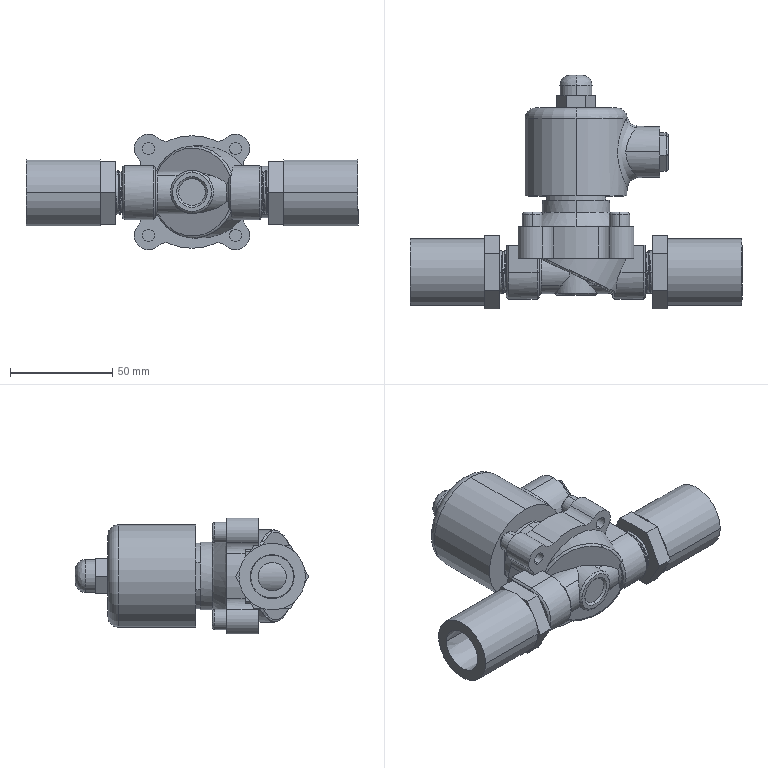Part | SolidWorks | 14 solids | 415 faces | box 162.238 x 114.123 x 56.5 mm | volume 232338 mm3 | cylinder 167 | plane 122 | cone 62 | spline 52 | torus 12 | commonest cylinder face diameters 19.583 x40 18.5 x37 45 x17 10 x16 6 x8 13.868 x8